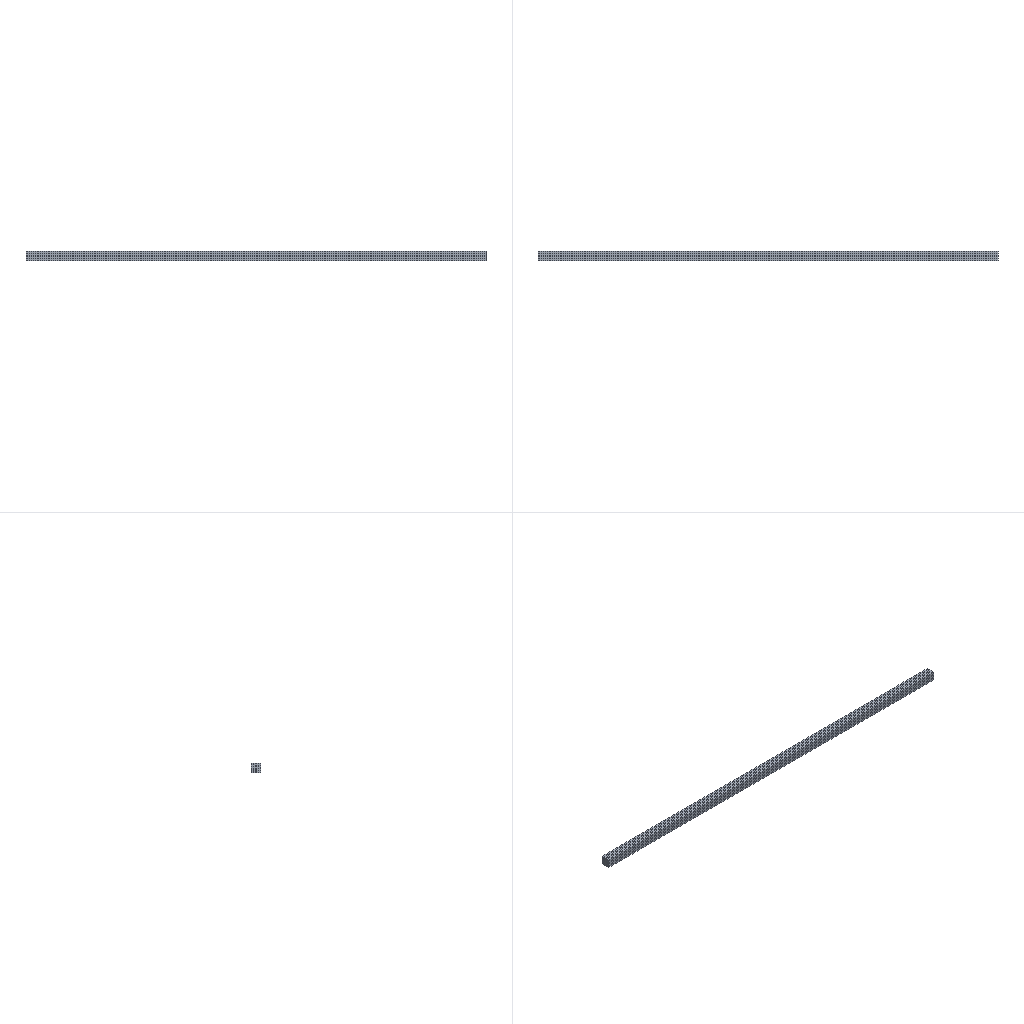Simulation study | ansys workbench
Set-up summary:
category,name,step,type,value,unit,region
solver,ansys_workbench
units,mm-N-s-tonne (MPa),,stated,"/units,MPA"
analysis,LS1,,static
load_step,LS1,LS1,static,nsubst=1; time=1
mesh,nodes,,,33096
mesh,elements,,,6250
element_type,SOLID186,,,6250
material,Structural Steel,,E,200000,tonne s^-2 mm^-1
material,Structural Steel,,nu,0.3
material,Structural Steel,,density,7.85e-09,tonne mm^-3
material,Structural Steel,,conductivity,60.5,tonne mm s^-3 C^-1
material,Structural Steel,,specific_heat,4.34e+08,mm^2 s^-2 C^-1
material,Structural Steel,,cte,1.2e-05,C^-1
material,Structural Steel,,permeability,10000
material,Structural Steel,,resistivity,0.00017,ohm mm
load,,LS1,pressure,-300,,all
load,ACEL,LS1,gravity (ACEL; gravity acts opposite),"9806.65 [dir=(0, -1, 0)]",,all
bc,Fixed Supports,model,fixed,[dofs=ALL],,_FIXEDSU
named_set,_FIXEDSU,,node,192
Ansys APDL input file, long lists of numbers shortened:
/batch
/config,noeldb,1     ! force off writing results to database
*get,_wallstrt,active,,time,wall
! ANSYS input file written by Workbench version 2021 R1
! File used for geometry attach:
/title,ansys___--____ (A5)
! ****** Begin Custom Load Command Snippet ******
/COM, ACT Extensions:
/COM,     LSDYNA, 2021.1
/COM,
! ****** End   Custom Load Command Snippet ******
*DIM,_wb_ProjectScratch_dir,string,248
_wb_ProjectScratch_dir(1) = ''
*DIM,_wb_SolverFiles_dir,string,248
_wb_SolverFiles_dir(1) = ''
*DIM,_wb_userfiles_dir,string,248
_wb_userfiles_dir(1) = ''
/com,--- Data in consistent NMM units. See Solving Units in the help system for more information.
/units,MPA
/nopr
/wb,file,start              !  signify a WB generated input file
/prep7
! Turn off shape checking because checks already performed inside WB mesher.
! See help system for more information.
SHPP,OFF,,NOWARN
/nolist
etcon,set             ! allow ANSYS to choose best KEYOP's for 180x elements, resets any applicable keyopt to MAPDL defaults
/com,*********** Nodes for the whole assembly ***********
nblock,3,,36405
(1i9,3e20.9e3)
        1     4.980000000E+03    -3.000000000E+01     3.000000000E+01
! (33095 more lines like these left out)
-1
/wb,elem,start            !  set before creation of elements
/com,*********** Elements for Body 1 "__5__-FreeParts|______3" ***********
et,1,186
keyo,1,2,1          ! set full integration on SOLID186
eblock,19,solid,,6250
(19i9)
        1        1        1        1        0        0        0        0       20        0        1        1     7742     8995     9000     4980     8738     8996     9016
! (12499 more lines like these left out)
-1
/wb,elem,end               !  done creating elements
/com,*********** Send User Defined Coordinate System(s) ***********
csys,0
toffst,273.15,  ! Temperature offset from absolute zero
/com,*********** Set Reference Temperature ***********
tref,22.
/wb,mat,start              !  starting to send materials
/com,*********** Send Materials ***********
Temperature = 'TEMP' ! Temperature
MP,DENS,1,7.85e-09,	! tonne mm^-3
MP,ALPX,1,1.2e-05,	! C^-1
MP,C,1,434000000,	! mm^2 s^-2 C^-1
MP,KXX,1,60.5,	! tonne mm s^-3 C^-1
MP,RSVX,1,0.00017,	! ohm mm
MP,EX,1,200000,	! tonne s^-2 mm^-1
MP,NUXY,1,0.3,
MP,MURX,1,10000,
/wb,mat,end                !  done sending materials
!************************* Model Summary ********************
!__5__-FreeParts|______3,	结构钢,	matid,	1
!************************* End Model Summary ********************
! get the diagonal of the bounding box. Needed later for other things
*get,_xmin,node,,mnloc,x
*get,_ymin,node,,mnloc,y
*get,_zmin,node,,mnloc,z
*get,_xmax,node,,mxloc,x
*get,_ymax,node,,mxloc,y
*get,_zmax,node,,mxloc,z
_ASMDIAG=(_xmax-_xmin)*(_xmax-_xmin)+(_ymax-_ymin)*(_ymax-_ymin)+(_zmax-_zmin)*(_zmax-_zmin)
_ASMDIAG=SQRT(_ASMDIAG)
/wb,contact,start          !  starting to send contact
/wb,contact,end            !  done creating contacts
/golist
/wb,load,start             !  starting to send loads
/com,*********** Fixed Supports ***********
CMBLOCK,_FIXEDSU,NODE,      192
(8i10)
      5977      5978      5979      5980      5981      5982      5983      5984
! (23 more lines like these left out)
cmsel,s,_FIXEDSU
d,all,all
nsel,all
/com,*********** Define Vertex Force Using Follower Elements ***********
et,2,201
keyo,2,1,1           ! Keep the direction constant
keyo,2,2,1           ! Apply Forces only, not moment
mat,2
real,2
type,2
en,11301,6865
r,2
rmod,2,1,1.0,              ! FX
mat,3
real,3
type,2
en,11302,6865
r,3
rmod,3,2,1.0,              ! FY
mat,4
real,4
type,2
en,11303,6865
r,4
rmod,4,3,1.0,              ! FZ
/gst,on,on
fini
*get,_numnode,node,0,count
*get,_numelem,elem,0,count
*get, _MAXELEMNUM, elem, 0, NUM, MAX
*get, _MAXNODENUM, node, 0, NUM, MAX
*get, _MAXELEMTYPE, etyp, 0, NUM, MAX
*get, _MAXREALCONST, real, 0, NUM, MAX
/go
/wb,load,end               !  done creating loads
/com,--- Number of total nodes = %_numnode%
/com,--- Number of contact elements = 0
/com,--- Number of spring elements = 0
/com,--- Number of bearing elements = 0
/com,--- Number of solid elements = 6250
/com,--- Number of condensed parts = 0
/com,--- Number of total elements = %_numelem%
*get,_wallbsol,active,,time,wall
/com,****************************************************************************
/com,*************************    SOLUTION       ********************************
/com,****************************************************************************
/solu
antype,0                   ! static analysis
_thickRatio=  1     ! Ratio of thick parts in the model
eqsl,pcg,1e-8,,,,,,1
cntr,print,1               ! print out contact info and also make no initial contact an error
dmpoption,emat,no             ! Don't combine emat file for DANSYS
dmpoption,esav,no             ! Don't combine esav file for DANSYS
nldiag,cont,iter           ! print out contact info each equilibrium iteration
rescontrol,,none                 ! Do not keep any restart files
/com,****************************************************
/com,******************* SOLVE FOR LS 1 OF 1 ****************
esel,s,real,,2
sfe,all,1,pres,1,0.
esel,s,real,,3
sfe,all,1,pres,1,-300.
esel,s,real,,4
sfe,all,1,pres,1,0.
esel,all
acel,0.,9806.65,0.
/nopr
/gopr
/nolist
nsub,1,1,1
time,1.
outres,erase
outres,all,none
outres,nsol,all,
outres,rsol,all
outres,eangl,all
outres,etmp,all
outres,veng,all
outres,strs,all,
outres,epel,all,
outres,eppl,all,
outres,cont,all,
! *********** WB SOLVE COMMAND ***********
! check interactive state
*get,ANSINTER_,active,,int
*if,ANSINTER_,ne,0,then
/eof
*endif
solve
/com *************** Write FE CONNECTORS *********
CEWRITE,file,ce,,INTE
/com,****************************************************
/com,*************** FINISHED SOLVE FOR LS 1 *************
*get,_wallasol,active,,time,wall
/nopr
*get,_numnode,node,0,count
*get,_numelem,elem,0,count
*get, _MAXELEMNUM, elem, 0, NUM, MAX
*get, _MAXNODENUM, node, 0, NUM, MAX,,,INTERNAL
*get, _MAXELEMTYPE, etyp, 0, NUM, MAX
*get, _MAXREALCONST, real, 0, NUM, MAX
/gopr
*get,_PCGITER,active,,solu,cgiter
/post1
xmlo,ENCODING,ISO-8859-1
xmlo,parm
/xml,parm,xml
fini
/gopr
*get,_walldone,active,,time,wall
_preptime=(_wallbsol-_wallstrt)*3600
_solvtime=(_wallasol-_wallbsol)*3600
_posttime=(_walldone-_wallasol)*3600
_totaltim=(_walldone-_wallstrt)*3600
*get,_dlbratio,active,0,solu,dlbr
*get,_combtime,active,0,solu,comb
/com,--- Total number of nodes = %_numnode%
/com,--- Total number of elements = %_numelem%
/com,--- Element load balance ratio = %_dlbratio%
/com,--- Time to combine distributed files = %_combtime%
/wb,file,end               ! done with WB generated input
Results summary:
result,analyses[0].index,,,1
result,analyses[0].system,,,SYS
result,analyses[0].deck,,,deck.dat
result,analyses[0].solve_status,,,completed
result,analyses[0].analysis_type,,,static
result,analyses[0].physics,,,mechanical
result,analyses[0].unit_system,,,"NMM: mm, ton, N, s, mV, mA, degC"
result,analyses[0].n_sets,,,1
result,analyses[0].load_steps[0].set,set=1,,1
result,analyses[0].load_steps[0].time_or_freq,set=1,,1
result,analyses[0].load_steps[0].max_displacement_magnitude,set=1,,0.87
result,analyses[0].load_steps[0].max_von_mises_nodal,set=1,,12.099
result,analyses[0].load_steps[0].reaction_force_sum_xyz[1],set=1,,-0.0004812
result,analyses[0].load_steps[0].reaction_force_sum_xyz[2],set=1,,4149.11
result,analyses[0].load_steps[0].reaction_force_sum_xyz[3],set=1,,-6.30811e-05
result,geometry_export[0][0],,,.step
result,geometry_export[0][1],,,ok
result,geometry_export[0][2],,,1